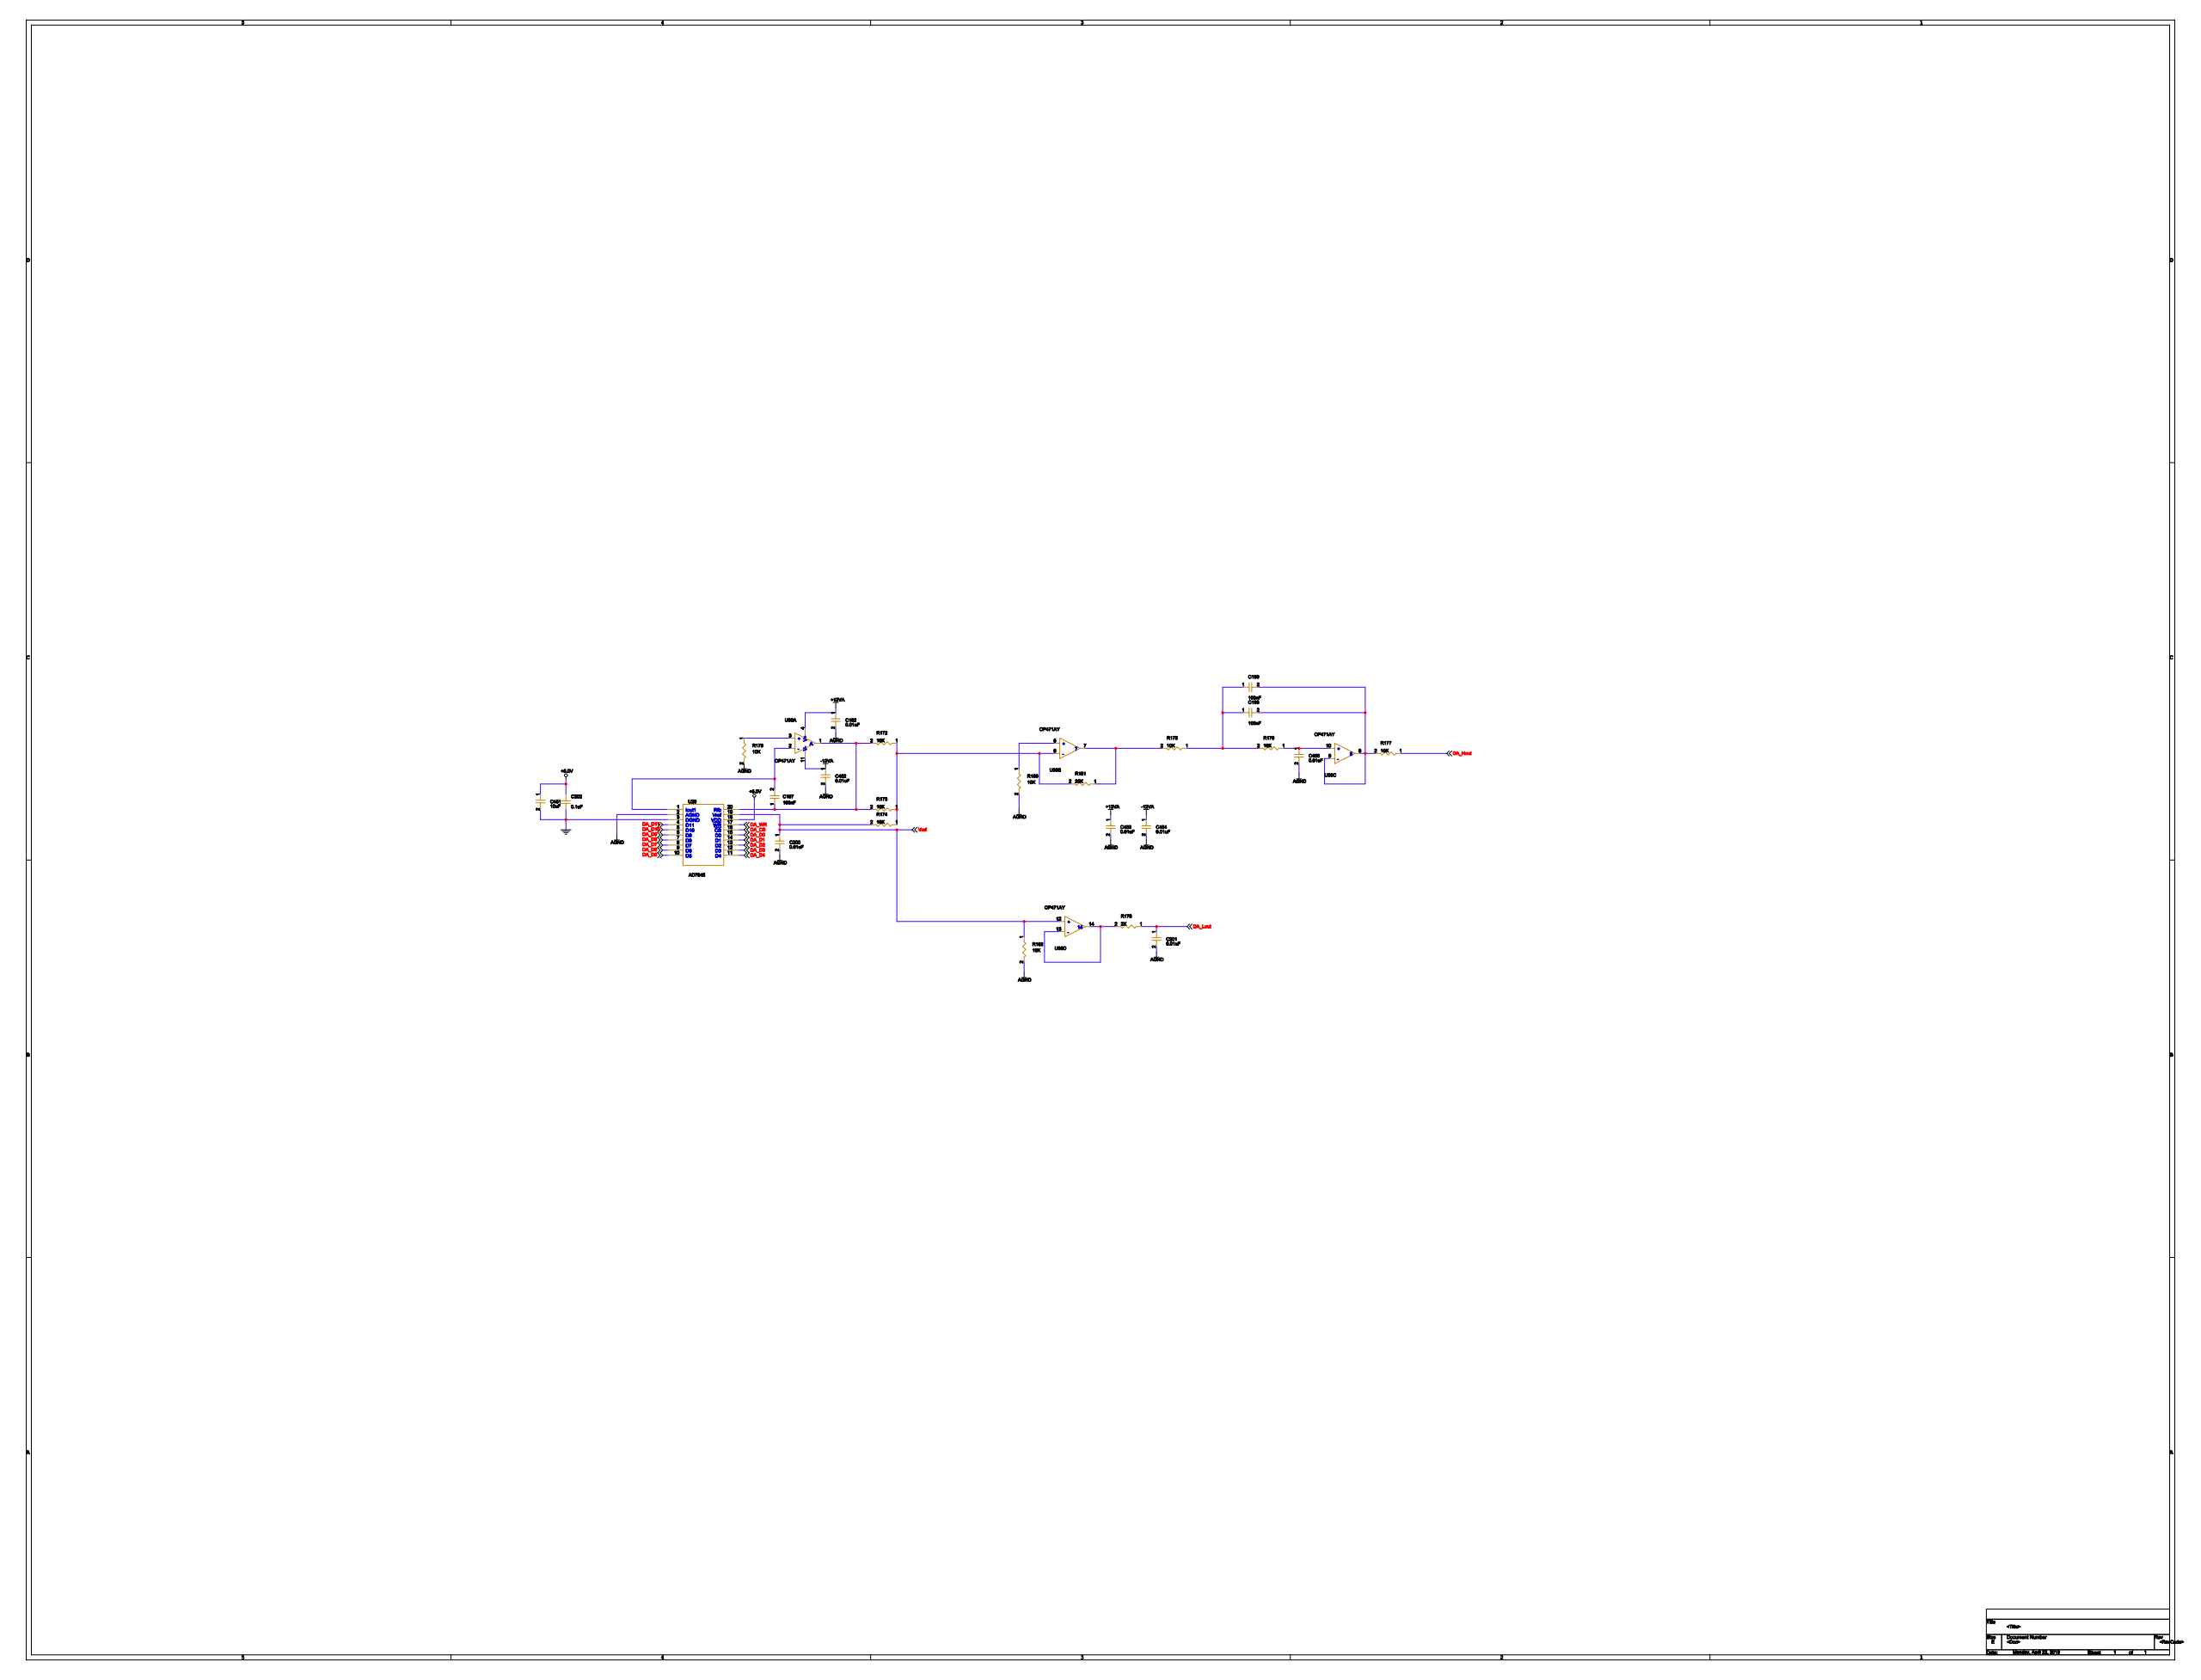Circuit board | Cadence Allegro | 362 parts | 391 nets | one sheet of the schematic
Parts on this sheet (reference | value | footprint):
C192 | 0.01uF | 1206
C197 | 100nF | 1206
C198 | 100nF | 1206
C199 | 100nF | 1206
C200 | 0.01uF | 1206
C201 | 0.01uF | 1206
C202 | 0.1uF | 1206
C451 | 10uF | 6032
C452 | 0.01uF | 1206
C453 | 0.01uF | 1206
C454 | 0.01uF | 1206
C455 | 0.01uF | 1206
R172 | 10K | 1206
R173 | 10K | 1206
R174 | 10K | 1206
R175 | 10K | 1206
R176 | 10K | 1206
R177 | 10K | 1206
R178 | 2K | 1206
R179 | 10K | 1206
R180 | 10K | 1206
R181 | 20K | 1206
R182 | 10K | 1206
U29 | AD7945 | TSSOP20
Nets of these parts (net: part-pin ...):
N17455227: R179-1
N17455852: C197-2 U29-1
N17455262: C197-1 R172-2 R173-2 U29-20
+12VA: C192-1 C453-1
-12VA: C452-1 C454-1
N17455274: R180-1
N17455288: R172-1 R173-1 R174-1 R181-2
N17455282: R175-2 R181-1
N17456727: C455-1 R176-1
N17456682: C198-2 C199-2 R177-2
VREF: C200-1 R174-2 R182-1 U29-19
N17455530: R178-2
DGND: C202-1 C451-2 U29-3
AGND: C192-2 C200-2 C201-2 C452-2 C453-2 C454-2 C455-2 R179-2 R180-2 R182-2 U29-2
DA_CS: U29-16
DA_D0: U29-15
DA_D1: U29-14
DA_D10: U29-5
DA_D11: U29-4
DA_D2: U29-13
DA_D3: U29-12
DA_D4: U29-11
DA_D5: U29-10
DA_D6: U29-9
DA_D7: U29-8
DA_D8: U29-7
DA_D9: U29-6
+5.0V: C202-2 C451-1 U29-18
DA_WR: U29-17
DA_HOUT: R177-1
DA_LOUT: C201-1 R178-1
N17456721: C198-1 C199-1 R175-1 R176-2